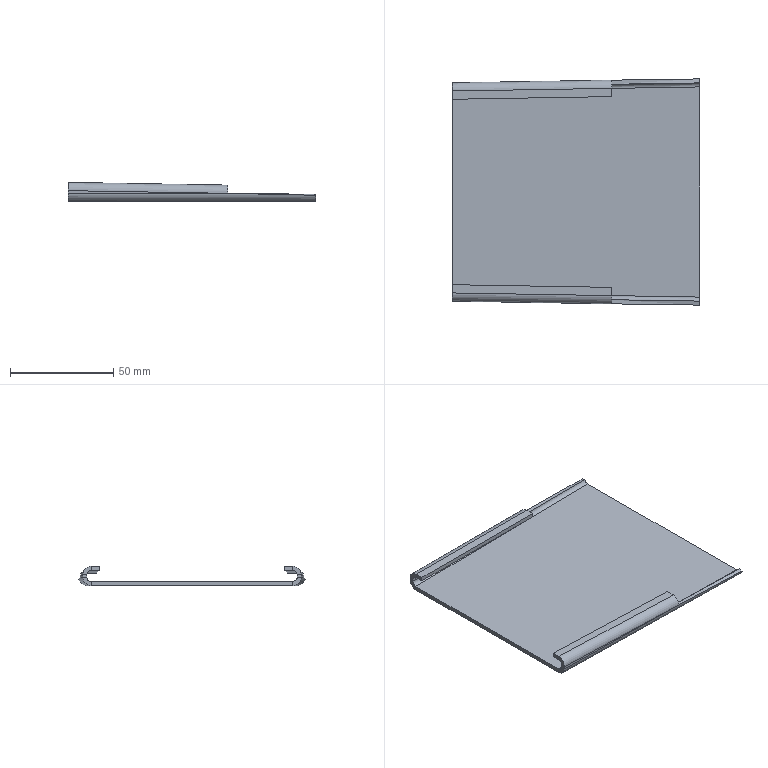Part | STEP file | A14-005 | 1 solid | 38 faces | box 120.042 x 109.776 x 9.287 mm | volume 29092 mm3 | plane 24 | cylinder 8 | spline 6 | commonest cylinder face diameters 4 x4 8 x4